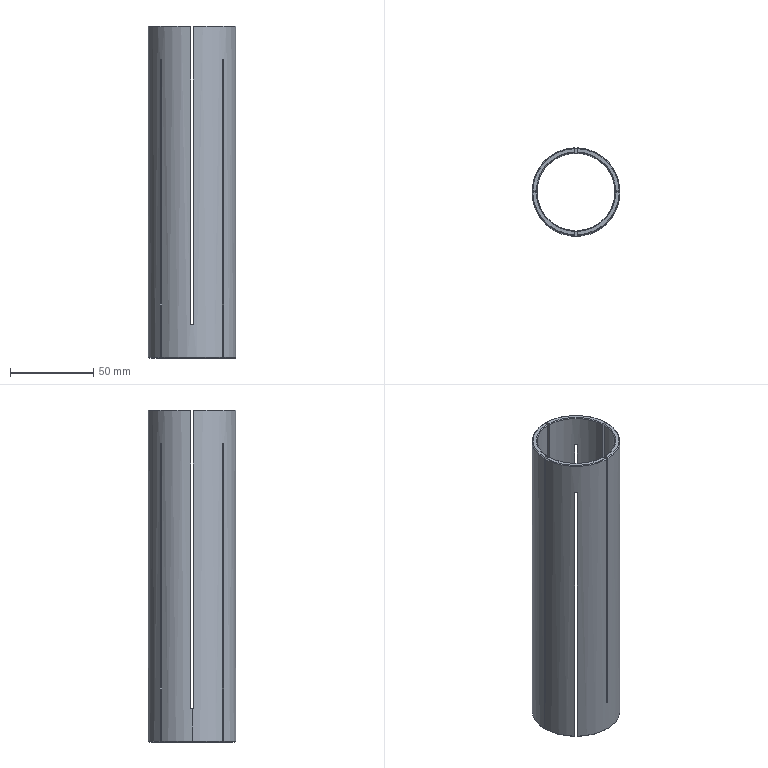Part | SolidWorks | features ICE 3, CirPattern 2, Chamfer 1, Extrusion 1, RefAxis 1 | 1 solid | 54 faces | box 53 x 53 x 200 mm | volume 87700 mm3 | plane 32 | cone 18 | cylinder 4 | commonest cylinder face diameters 47 x2 53 x2